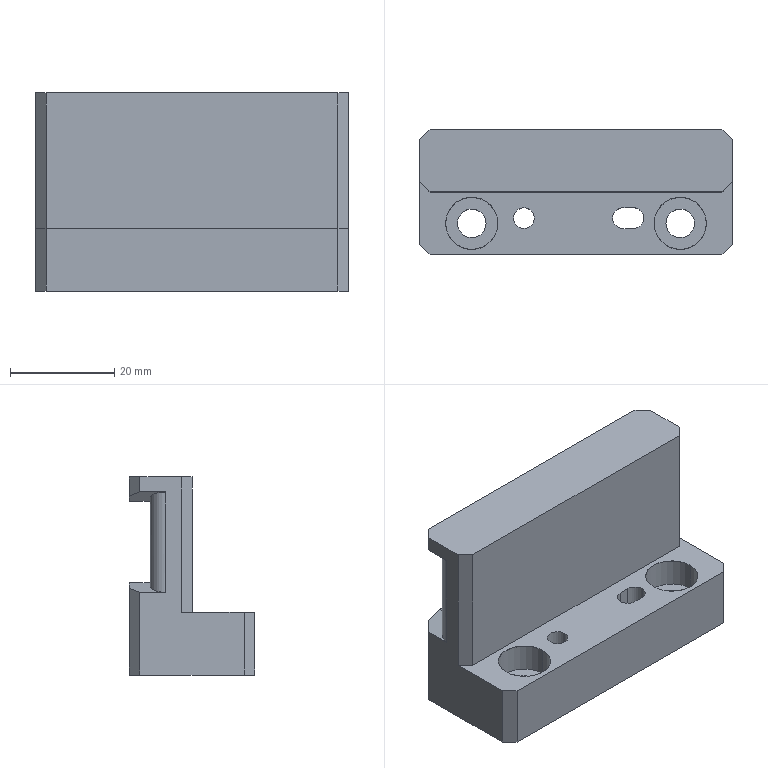Part | STEP file | QA-AD11 | 1 solid | 47 faces | box 60 x 24 x 38 mm | volume 30322 mm3 | plane 28 | cylinder 15 | cone 4 | commonest cylinder face diameters 4 x5 5.5 x4 10 x4 6 x2